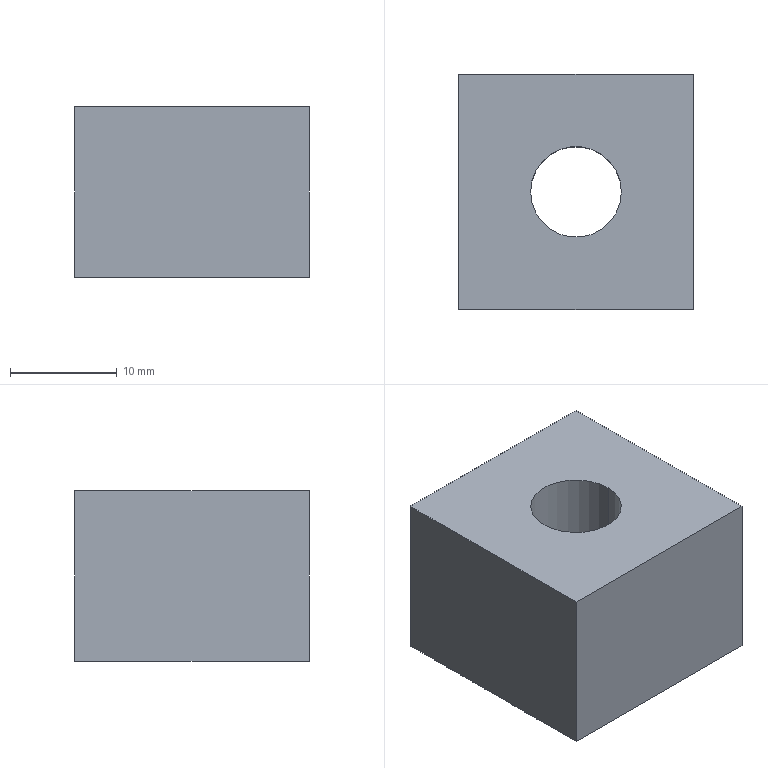Part | SolidWorks | features Extrusion 1, HoleWzd 1 | 1 solid | 8 faces | box 22 x 22 x 16 mm | volume 6836 mm3 | plane 6 | cylinder 2 | commonest cylinder face diameters 8.5 x2
STEP:
#1=CARTESIAN_POINT('',(-4.25,0.,0.));
#2=VERTEX_POINT('',#1);
#3=CARTESIAN_POINT('',(4.25,0.,0.));
#4=VERTEX_POINT('',#3);
#5=CARTESIAN_POINT('',(0.,0.,0.));
#6=DIRECTION('',(0.,0.,1.));
#7=DIRECTION('',(1.,0.,0.));
#8=AXIS2_PLACEMENT_3D('',#5,#6,#7);
#9=CIRCLE('',#8,4.25);
#10=EDGE_CURVE('',#2,#4,#9,.T.);
#11=ORIENTED_EDGE('',*,*,#10,.F.);
#12=CARTESIAN_POINT('',(-4.25,0.,16.));
#13=VERTEX_POINT('',#12);
#14=CARTESIAN_POINT('',(-4.25,0.,16.));
#15=DIRECTION('',(0.,0.,1.));
#16=VECTOR('',#15,1000.);
#17=LINE('',#14,#16);
#18=EDGE_CURVE('',#2,#13,#17,.T.);
#19=ORIENTED_EDGE('',*,*,#18,.T.);
#20=CARTESIAN_POINT('',(4.25,0.,16.));
#21=VERTEX_POINT('',#20);
#22=CARTESIAN_POINT('',(0.,0.,16.));
#23=DIRECTION('',(0.,0.,1.));
#24=DIRECTION('',(1.,0.,0.));
#25=AXIS2_PLACEMENT_3D('',#22,#23,#24);
#26=CIRCLE('',#25,4.25);
#27=EDGE_CURVE('',#13,#21,#26,.T.);
#28=ORIENTED_EDGE('',*,*,#27,.T.);
#29=CARTESIAN_POINT('',(4.25,0.,16.));
#30=DIRECTION('',(0.,0.,1.));
#31=VECTOR('',#30,1000.);
#32=LINE('',#29,#31);
#33=EDGE_CURVE('',#4,#21,#32,.T.);
#34=ORIENTED_EDGE('',*,*,#33,.F.);
#35=EDGE_LOOP('',(#11,#19,#28,#34));
#36=FACE_OUTER_BOUND('',#35,.T.);
#37=CARTESIAN_POINT('',(0.,0.,16.));
#38=DIRECTION('',(0.,0.,1.));
#39=DIRECTION('',(1.,0.,0.));
#40=AXIS2_PLACEMENT_3D('',#37,#38,#39);
#41=CYLINDRICAL_SURFACE('',#40,4.25);
#42=ADVANCED_FACE('',(#36),#41,.F.);
#43=CARTESIAN_POINT('',(11.,-11.,0.));
#44=VERTEX_POINT('',#43);
#45=CARTESIAN_POINT('',(11.,11.,0.));
#46=VERTEX_POINT('',#45);
#47=CARTESIAN_POINT('',(11.,11.,0.));
#48=DIRECTION('',(0.,1.,0.));
#49=VECTOR('',#48,1000.);
#50=LINE('',#47,#49);
#51=EDGE_CURVE('',#44,#46,#50,.T.);
#52=ORIENTED_EDGE('',*,*,#51,.T.);
#53=CARTESIAN_POINT('',(11.,11.,16.));
#54=VERTEX_POINT('',#53);
#55=CARTESIAN_POINT('',(11.,11.,16.));
#56=DIRECTION('',(0.,0.,-1.));
#57=VECTOR('',#56,1000.);
#58=LINE('',#55,#57);
#59=EDGE_CURVE('',#54,#46,#58,.T.);
#60=ORIENTED_EDGE('',*,*,#59,.F.);
#61=CARTESIAN_POINT('',(11.,-11.,16.));
#62=VERTEX_POINT('',#61);
#63=CARTESIAN_POINT('',(11.,11.,16.));
#64=DIRECTION('',(0.,1.,0.));
#65=VECTOR('',#64,1000.);
#66=LINE('',#63,#65);
#67=EDGE_CURVE('',#62,#54,#66,.T.);
#68=ORIENTED_EDGE('',*,*,#67,.F.);
#69=CARTESIAN_POINT('',(11.,-11.,16.));
#70=DIRECTION('',(0.,0.,-1.));
#71=VECTOR('',#70,1000.);
#72=LINE('',#69,#71);
#73=EDGE_CURVE('',#62,#44,#72,.T.);
#74=ORIENTED_EDGE('',*,*,#73,.T.);
#75=EDGE_LOOP('',(#52,#60,#68,#74));
#76=FACE_OUTER_BOUND('',#75,.T.);
#77=CARTESIAN_POINT('',(11.,11.,16.));
#78=DIRECTION('',(-1.,0.,0.));
#79=DIRECTION('',(0.,-1.,0.));
#80=AXIS2_PLACEMENT_3D('',#77,#78,#79);
#81=PLANE('',#80);
#82=ADVANCED_FACE('',(#76),#81,.F.);
#83=CARTESIAN_POINT('',(-11.,11.,0.));
#84=VERTEX_POINT('',#83);
#85=CARTESIAN_POINT('',(-11.,11.,0.));
#86=DIRECTION('',(-1.,0.,0.));
#87=VECTOR('',#86,1000.);
#88=LINE('',#85,#87);
#89=EDGE_CURVE('',#46,#84,#88,.T.);
#90=ORIENTED_EDGE('',*,*,#89,.T.);
#91=CARTESIAN_POINT('',(-11.,11.,16.));
#92=VERTEX_POINT('',#91);
#93=CARTESIAN_POINT('',(-11.,11.,16.));
#94=DIRECTION('',(0.,0.,-1.));
#95=VECTOR('',#94,1000.);
#96=LINE('',#93,#95);
#97=EDGE_CURVE('',#92,#84,#96,.T.);
#98=ORIENTED_EDGE('',*,*,#97,.F.);
#99=CARTESIAN_POINT('',(-11.,11.,16.));
#100=DIRECTION('',(-1.,0.,0.));
#101=VECTOR('',#100,1000.);
#102=LINE('',#99,#101);
#103=EDGE_CURVE('',#54,#92,#102,.T.);
#104=ORIENTED_EDGE('',*,*,#103,.F.);
#105=ORIENTED_EDGE('',*,*,#59,.T.);
#106=EDGE_LOOP('',(#90,#98,#104,#105));
#107=FACE_OUTER_BOUND('',#106,.T.);
#108=CARTESIAN_POINT('',(-11.,11.,16.));
#109=DIRECTION('',(0.,-1.,0.));
#110=DIRECTION('',(0.,0.,-1.));
#111=AXIS2_PLACEMENT_3D('',#108,#109,#110);
#112=PLANE('',#111);
#113=ADVANCED_FACE('',(#107),#112,.F.);
#114=CARTESIAN_POINT('',(-11.,-11.,0.));
#115=VERTEX_POINT('',#114);
#116=CARTESIAN_POINT('',(-11.,11.,0.));
#117=DIRECTION('',(0.,-1.,0.));
#118=VECTOR('',#117,1000.);
#119=LINE('',#116,#118);
#120=EDGE_CURVE('',#84,#115,#119,.T.);
#121=ORIENTED_EDGE('',*,*,#120,.T.);
#122=CARTESIAN_POINT('',(-11.,-11.,16.));
#123=VERTEX_POINT('',#122);
#124=CARTESIAN_POINT('',(-11.,-11.,16.));
#125=DIRECTION('',(0.,0.,-1.));
#126=VECTOR('',#125,1000.);
#127=LINE('',#124,#126);
#128=EDGE_CURVE('',#123,#115,#127,.T.);
#129=ORIENTED_EDGE('',*,*,#128,.F.);
#130=CARTESIAN_POINT('',(-11.,11.,16.));
#131=DIRECTION('',(0.,-1.,0.));
#132=VECTOR('',#131,1000.);
#133=LINE('',#130,#132);
#134=EDGE_CURVE('',#92,#123,#133,.T.);
#135=ORIENTED_EDGE('',*,*,#134,.F.);
#136=ORIENTED_EDGE('',*,*,#97,.T.);
#137=EDGE_LOOP('',(#121,#129,#135,#136));
#138=FACE_OUTER_BOUND('',#137,.T.);
#139=CARTESIAN_POINT('',(-11.,11.,16.));
#140=DIRECTION('',(1.,0.,0.));
#141=DIRECTION('',(0.,1.,0.));
#142=AXIS2_PLACEMENT_3D('',#139,#140,#141);
#143=PLANE('',#142);
#144=ADVANCED_FACE('',(#138),#143,.F.);
#145=CARTESIAN_POINT('',(-11.,-11.,0.));
#146=DIRECTION('',(1.,0.,0.));
#147=VECTOR('',#146,1000.);
#148=LINE('',#145,#147);
#149=EDGE_CURVE('',#115,#44,#148,.T.);
#150=ORIENTED_EDGE('',*,*,#149,.T.);
#151=ORIENTED_EDGE('',*,*,#73,.F.);
#152=CARTESIAN_POINT('',(-11.,-11.,16.));
#153=DIRECTION('',(1.,0.,0.));
#154=VECTOR('',#153,1000.);
#155=LINE('',#152,#154);
#156=EDGE_CURVE('',#123,#62,#155,.T.);
#157=ORIENTED_EDGE('',*,*,#156,.F.);
#158=ORIENTED_EDGE('',*,*,#128,.T.);
#159=EDGE_LOOP('',(#150,#151,#157,#158));
#160=FACE_OUTER_BOUND('',#159,.T.);
#161=CARTESIAN_POINT('',(-11.,-11.,16.));
#162=DIRECTION('',(0.,1.,0.));
#163=DIRECTION('',(0.,0.,1.));
#164=AXIS2_PLACEMENT_3D('',#161,#162,#163);
#165=PLANE('',#164);
#166=ADVANCED_FACE('',(#160),#165,.F.);
#167=CARTESIAN_POINT('',(0.,0.,16.));
#168=DIRECTION('',(0.,0.,1.));
#169=DIRECTION('',(1.,0.,0.));
#170=AXIS2_PLACEMENT_3D('',#167,#168,#169);
#171=CIRCLE('',#170,4.25);
#172=EDGE_CURVE('',#21,#13,#171,.T.);
#173=ORIENTED_EDGE('',*,*,#172,.F.);
#174=ORIENTED_EDGE('',*,*,#27,.F.);
#175=EDGE_LOOP('',(#173,#174));
#176=FACE_BOUND('',#175,.T.);
#177=ORIENTED_EDGE('',*,*,#67,.T.);
#178=ORIENTED_EDGE('',*,*,#103,.T.);
#179=ORIENTED_EDGE('',*,*,#134,.T.);
#180=ORIENTED_EDGE('',*,*,#156,.T.);
#181=EDGE_LOOP('',(#177,#178,#179,#180));
#182=FACE_OUTER_BOUND('',#181,.T.);
#183=CARTESIAN_POINT('',(0.,0.,16.));
#184=DIRECTION('',(0.,0.,1.));
#185=DIRECTION('',(1.,0.,0.));
#186=AXIS2_PLACEMENT_3D('',#183,#184,#185);
#187=PLANE('',#186);
#188=ADVANCED_FACE('',(#176,#182),#187,.T.);
#189=CARTESIAN_POINT('',(0.,0.,0.));
#190=DIRECTION('',(0.,0.,1.));
#191=DIRECTION('',(1.,0.,0.));
#192=AXIS2_PLACEMENT_3D('',#189,#190,#191);
#193=CIRCLE('',#192,4.25);
#194=EDGE_CURVE('',#4,#2,#193,.T.);
#195=ORIENTED_EDGE('',*,*,#194,.T.);
#196=ORIENTED_EDGE('',*,*,#10,.T.);
#197=EDGE_LOOP('',(#195,#196));
#198=FACE_BOUND('',#197,.T.);
#199=ORIENTED_EDGE('',*,*,#51,.F.);
#200=ORIENTED_EDGE('',*,*,#149,.F.);
#201=ORIENTED_EDGE('',*,*,#120,.F.);
#202=ORIENTED_EDGE('',*,*,#89,.F.);
#203=EDGE_LOOP('',(#199,#200,#201,#202));
#204=FACE_OUTER_BOUND('',#203,.T.);
#205=CARTESIAN_POINT('',(0.,0.,0.));
#206=DIRECTION('',(0.,0.,1.));
#207=DIRECTION('',(1.,0.,0.));
#208=AXIS2_PLACEMENT_3D('',#205,#206,#207);
#209=PLANE('',#208);
#210=ADVANCED_FACE('',(#198,#204),#209,.F.);
#211=ORIENTED_EDGE('',*,*,#18,.F.);
#212=ORIENTED_EDGE('',*,*,#194,.F.);
#213=ORIENTED_EDGE('',*,*,#33,.T.);
#214=ORIENTED_EDGE('',*,*,#172,.T.);
#215=EDGE_LOOP('',(#211,#212,#213,#214));
#216=FACE_OUTER_BOUND('',#215,.T.);
#217=CARTESIAN_POINT('',(0.,0.,16.));
#218=DIRECTION('',(0.,0.,1.));
#219=DIRECTION('',(1.,0.,0.));
#220=AXIS2_PLACEMENT_3D('',#217,#218,#219);
#221=CYLINDRICAL_SURFACE('',#220,4.25);
#222=ADVANCED_FACE('',(#216),#221,.F.);
#223=CLOSED_SHELL('',(#42,#82,#113,#144,#166,#188,#210,#222));
#224=MANIFOLD_SOLID_BREP('',#223);
#225=CARTESIAN_POINT('',(0.,0.,0.));
#226=DIRECTION('',(0.,0.,1.));
#227=DIRECTION('',(1.,0.,0.));
#228=AXIS2_PLACEMENT_3D('',#225,#226,#227);
#229=(LENGTH_UNIT()NAMED_UNIT(*)SI_UNIT(.MILLI.,.METRE.));
#230=UNCERTAINTY_MEASURE_WITH_UNIT(LENGTH_MEASURE(0.00001),#229,'','');
#231=(NAMED_UNIT(*)PLANE_ANGLE_UNIT()SI_UNIT($,.RADIAN.));
#232=(NAMED_UNIT(*)SI_UNIT($,.STERADIAN.)SOLID_ANGLE_UNIT());
#233=(GEOMETRIC_REPRESENTATION_CONTEXT(3)GLOBAL_UNCERTAINTY_ASSIGNED_CONTEXT((#230))GLOBAL_UNIT_ASSIGNED_CONTEXT((#229,#231,#232))REPRESENTATION_CONTEXT('',''));
#234=ADVANCED_BREP_SHAPE_REPRESENTATION('',(#224,#228),#233);